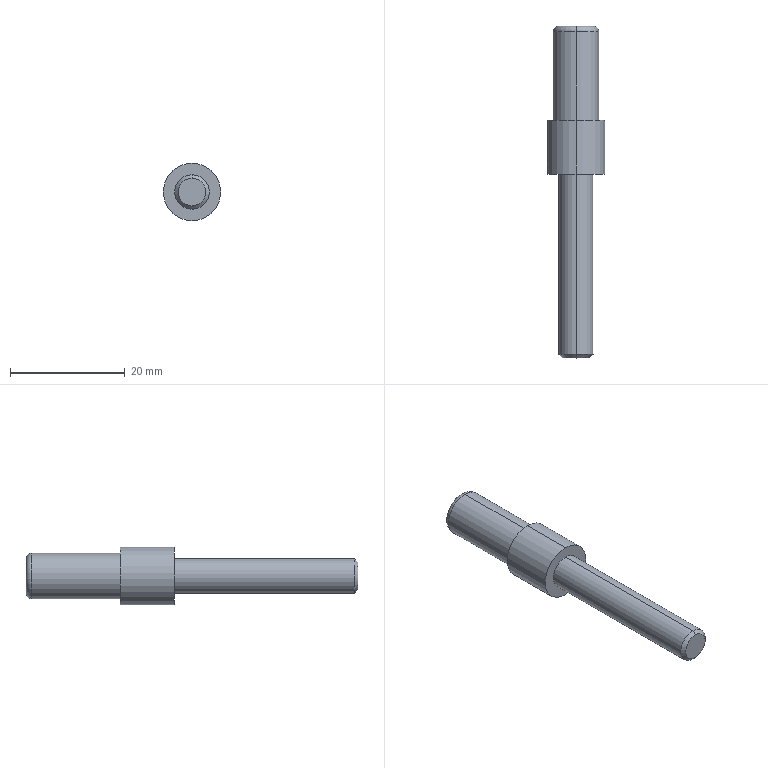Part | SolidWorks | features RefAxis 3, 3DProfileFeature 1, ICE 1, Revolution 1 | 1 solid | 21 faces | box 10 x 57.8 x 10 mm | volume 2436 mm3 | plane 11 | cylinder 6 | cone 2 | torus 2 | commonest cylinder face diameters 6 x2 8 x2 10 x2
STEP:
#1=CARTESIAN_POINT('',(0.,-32.,2.386));
#2=VERTEX_POINT('',#1);
#3=CARTESIAN_POINT('',(0.,-32.,-2.386));
#4=VERTEX_POINT('',#3);
#5=CARTESIAN_POINT('',(0.,-32.,0.));
#6=DIRECTION('',(0.,1.,0.));
#7=DIRECTION('',(0.,0.,1.));
#8=AXIS2_PLACEMENT_3D('',#5,#6,#7);
#9=CIRCLE('',#8,2.386);
#10=EDGE_CURVE('',#2,#4,#9,.T.);
#11=ORIENTED_EDGE('',*,*,#10,.T.);
#12=CARTESIAN_POINT('',(0.,-31.386,-3.));
#13=VERTEX_POINT('',#12);
#14=CARTESIAN_POINT('',(0.,-32.,-2.386));
#15=DIRECTION('',(0.,0.7071,-0.7071));
#16=VECTOR('',#15,1000.);
#17=LINE('',#14,#16);
#18=EDGE_CURVE('',#4,#13,#17,.T.);
#19=ORIENTED_EDGE('',*,*,#18,.T.);
#20=CARTESIAN_POINT('',(0.,-31.386,3.));
#21=VERTEX_POINT('',#20);
#22=CARTESIAN_POINT('',(0.,-31.386,0.));
#23=DIRECTION('',(0.,1.,0.));
#24=DIRECTION('',(0.,0.,1.));
#25=AXIS2_PLACEMENT_3D('',#22,#23,#24);
#26=CIRCLE('',#25,3.);
#27=EDGE_CURVE('',#21,#13,#26,.T.);
#28=ORIENTED_EDGE('',*,*,#27,.F.);
#29=CARTESIAN_POINT('',(0.,-32.,2.386));
#30=DIRECTION('',(0.,0.7071,0.7071));
#31=VECTOR('',#30,1000.);
#32=LINE('',#29,#31);
#33=EDGE_CURVE('',#2,#21,#32,.T.);
#34=ORIENTED_EDGE('',*,*,#33,.F.);
#35=EDGE_LOOP('',(#11,#19,#28,#34));
#36=FACE_OUTER_BOUND('',#35,.T.);
#37=CARTESIAN_POINT('',(0.,-32.,0.));
#38=DIRECTION('',(0.,1.,0.));
#39=DIRECTION('',(0.,0.,1.));
#40=AXIS2_PLACEMENT_3D('',#37,#38,#39);
#41=CONICAL_SURFACE('',#40,2.386,0.7854);
#42=ADVANCED_FACE('',(#36),#41,.T.);
#43=ORIENTED_EDGE('',*,*,#27,.T.);
#44=CARTESIAN_POINT('',(0.,0.,-3.));
#45=VERTEX_POINT('',#44);
#46=CARTESIAN_POINT('',(0.,-32.,-3.));
#47=DIRECTION('',(0.,1.,0.));
#48=VECTOR('',#47,1000.);
#49=LINE('',#46,#48);
#50=EDGE_CURVE('',#13,#45,#49,.T.);
#51=ORIENTED_EDGE('',*,*,#50,.T.);
#52=CARTESIAN_POINT('',(0.,0.,3.));
#53=VERTEX_POINT('',#52);
#54=CARTESIAN_POINT('',(0.,0.,0.));
#55=DIRECTION('',(0.,1.,0.));
#56=DIRECTION('',(0.,0.,1.));
#57=AXIS2_PLACEMENT_3D('',#54,#55,#56);
#58=CIRCLE('',#57,3.);
#59=EDGE_CURVE('',#53,#45,#58,.T.);
#60=ORIENTED_EDGE('',*,*,#59,.F.);
#61=CARTESIAN_POINT('',(0.,-32.,3.));
#62=DIRECTION('',(0.,1.,0.));
#63=VECTOR('',#62,1000.);
#64=LINE('',#61,#63);
#65=EDGE_CURVE('',#21,#53,#64,.T.);
#66=ORIENTED_EDGE('',*,*,#65,.F.);
#67=EDGE_LOOP('',(#43,#51,#60,#66));
#68=FACE_OUTER_BOUND('',#67,.T.);
#69=CARTESIAN_POINT('',(0.,-32.,0.));
#70=DIRECTION('',(0.,1.,0.));
#71=DIRECTION('',(0.,0.,1.));
#72=AXIS2_PLACEMENT_3D('',#69,#70,#71);
#73=CYLINDRICAL_SURFACE('',#72,3.);
#74=ADVANCED_FACE('',(#68),#73,.T.);
#75=CARTESIAN_POINT('',(0.,0.,5.));
#76=VERTEX_POINT('',#75);
#77=CARTESIAN_POINT('',(0.,0.,-5.));
#78=VERTEX_POINT('',#77);
#79=CARTESIAN_POINT('',(0.,0.,0.));
#80=DIRECTION('',(0.,1.,0.));
#81=DIRECTION('',(0.,0.,1.));
#82=AXIS2_PLACEMENT_3D('',#79,#80,#81);
#83=CIRCLE('',#82,5.);
#84=EDGE_CURVE('',#76,#78,#83,.T.);
#85=ORIENTED_EDGE('',*,*,#84,.T.);
#86=CARTESIAN_POINT('',(0.,9.4,-5.));
#87=VERTEX_POINT('',#86);
#88=CARTESIAN_POINT('',(0.,-32.,-5.));
#89=DIRECTION('',(0.,1.,0.));
#90=VECTOR('',#89,1000.);
#91=LINE('',#88,#90);
#92=EDGE_CURVE('',#78,#87,#91,.T.);
#93=ORIENTED_EDGE('',*,*,#92,.T.);
#94=CARTESIAN_POINT('',(0.,9.4,5.));
#95=VERTEX_POINT('',#94);
#96=CARTESIAN_POINT('',(0.,9.4,0.));
#97=DIRECTION('',(0.,1.,0.));
#98=DIRECTION('',(0.,0.,1.));
#99=AXIS2_PLACEMENT_3D('',#96,#97,#98);
#100=CIRCLE('',#99,5.);
#101=EDGE_CURVE('',#95,#87,#100,.T.);
#102=ORIENTED_EDGE('',*,*,#101,.F.);
#103=CARTESIAN_POINT('',(0.,-32.,5.));
#104=DIRECTION('',(0.,1.,0.));
#105=VECTOR('',#104,1000.);
#106=LINE('',#103,#105);
#107=EDGE_CURVE('',#76,#95,#106,.T.);
#108=ORIENTED_EDGE('',*,*,#107,.F.);
#109=EDGE_LOOP('',(#85,#93,#102,#108));
#110=FACE_OUTER_BOUND('',#109,.T.);
#111=CARTESIAN_POINT('',(0.,-32.,0.));
#112=DIRECTION('',(0.,1.,0.));
#113=DIRECTION('',(0.,0.,1.));
#114=AXIS2_PLACEMENT_3D('',#111,#112,#113);
#115=CYLINDRICAL_SURFACE('',#114,5.);
#116=ADVANCED_FACE('',(#110),#115,.T.);
#117=CARTESIAN_POINT('',(0.,9.4,4.));
#118=VERTEX_POINT('',#117);
#119=CARTESIAN_POINT('',(0.,9.4,-4.));
#120=VERTEX_POINT('',#119);
#121=CARTESIAN_POINT('',(0.,9.4,0.));
#122=DIRECTION('',(0.,1.,0.));
#123=DIRECTION('',(0.,0.,1.));
#124=AXIS2_PLACEMENT_3D('',#121,#122,#123);
#125=CIRCLE('',#124,4.);
#126=EDGE_CURVE('',#118,#120,#125,.T.);
#127=ORIENTED_EDGE('',*,*,#126,.T.);
#128=CARTESIAN_POINT('',(0.,24.8,-4.));
#129=VERTEX_POINT('',#128);
#130=CARTESIAN_POINT('',(0.,-32.,-4.));
#131=DIRECTION('',(0.,1.,0.));
#132=VECTOR('',#131,1000.);
#133=LINE('',#130,#132);
#134=EDGE_CURVE('',#120,#129,#133,.T.);
#135=ORIENTED_EDGE('',*,*,#134,.T.);
#136=CARTESIAN_POINT('',(0.,24.8,4.));
#137=VERTEX_POINT('',#136);
#138=CARTESIAN_POINT('',(0.,24.8,0.));
#139=DIRECTION('',(0.,1.,0.));
#140=DIRECTION('',(0.,0.,1.));
#141=AXIS2_PLACEMENT_3D('',#138,#139,#140);
#142=CIRCLE('',#141,4.);
#143=EDGE_CURVE('',#137,#129,#142,.T.);
#144=ORIENTED_EDGE('',*,*,#143,.F.);
#145=CARTESIAN_POINT('',(0.,-32.,4.));
#146=DIRECTION('',(0.,1.,0.));
#147=VECTOR('',#146,1000.);
#148=LINE('',#145,#147);
#149=EDGE_CURVE('',#118,#137,#148,.T.);
#150=ORIENTED_EDGE('',*,*,#149,.F.);
#151=EDGE_LOOP('',(#127,#135,#144,#150));
#152=FACE_OUTER_BOUND('',#151,.T.);
#153=CARTESIAN_POINT('',(0.,-32.,0.));
#154=DIRECTION('',(0.,1.,0.));
#155=DIRECTION('',(0.,0.,1.));
#156=AXIS2_PLACEMENT_3D('',#153,#154,#155);
#157=CYLINDRICAL_SURFACE('',#156,4.);
#158=ADVANCED_FACE('',(#152),#157,.T.);
#159=ORIENTED_EDGE('',*,*,#143,.T.);
#160=CARTESIAN_POINT('',(0.,25.8,-3.));
#161=VERTEX_POINT('',#160);
#162=CARTESIAN_POINT('',(0.,24.8,-3.));
#163=DIRECTION('',(1.,0.,0.));
#164=DIRECTION('',(0.,0.,-1.));
#165=AXIS2_PLACEMENT_3D('',#162,#163,#164);
#166=CIRCLE('',#165,1.);
#167=EDGE_CURVE('',#129,#161,#166,.T.);
#168=ORIENTED_EDGE('',*,*,#167,.T.);
#169=CARTESIAN_POINT('',(0.,25.8,3.));
#170=VERTEX_POINT('',#169);
#171=CARTESIAN_POINT('',(0.,25.8,0.));
#172=DIRECTION('',(0.,1.,0.));
#173=DIRECTION('',(0.,0.,1.));
#174=AXIS2_PLACEMENT_3D('',#171,#172,#173);
#175=CIRCLE('',#174,3.);
#176=EDGE_CURVE('',#170,#161,#175,.T.);
#177=ORIENTED_EDGE('',*,*,#176,.F.);
#178=CARTESIAN_POINT('',(0.,24.8,3.));
#179=DIRECTION('',(-1.,0.,0.));
#180=DIRECTION('',(0.,0.,1.));
#181=AXIS2_PLACEMENT_3D('',#178,#179,#180);
#182=CIRCLE('',#181,1.);
#183=EDGE_CURVE('',#137,#170,#182,.T.);
#184=ORIENTED_EDGE('',*,*,#183,.F.);
#185=EDGE_LOOP('',(#159,#168,#177,#184));
#186=FACE_OUTER_BOUND('',#185,.T.);
#187=CARTESIAN_POINT('',(0.,24.8,0.));
#188=DIRECTION('',(0.,1.,0.));
#189=DIRECTION('',(0.,0.,1.));
#190=AXIS2_PLACEMENT_3D('',#187,#188,#189);
#191=TOROIDAL_SURFACE('',#190,3.,1.);
#192=ADVANCED_FACE('',(#186),#191,.T.);
#193=CARTESIAN_POINT('',(-1.5,25.8,0.866));
#194=VERTEX_POINT('',#193);
#195=CARTESIAN_POINT('',(-1.5,25.8,-0.866));
#196=VERTEX_POINT('',#195);
#197=CARTESIAN_POINT('',(-1.5,25.8,0.));
#198=DIRECTION('',(0.,0.,-1.));
#199=VECTOR('',#198,1000.);
#200=LINE('',#197,#199);
#201=EDGE_CURVE('',#194,#196,#200,.T.);
#202=ORIENTED_EDGE('',*,*,#201,.T.);
#203=CARTESIAN_POINT('',(0.,25.8,-1.732));
#204=VERTEX_POINT('',#203);
#205=CARTESIAN_POINT('',(-0.75,25.8,-1.299));
#206=DIRECTION('',(0.866,0.,-0.5));
#207=VECTOR('',#206,1000.);
#208=LINE('',#205,#207);
#209=EDGE_CURVE('',#196,#204,#208,.T.);
#210=ORIENTED_EDGE('',*,*,#209,.T.);
#211=CARTESIAN_POINT('',(1.5,25.8,-0.866));
#212=VERTEX_POINT('',#211);
#213=CARTESIAN_POINT('',(0.75,25.8,-1.299));
#214=DIRECTION('',(0.866,0.,0.5));
#215=VECTOR('',#214,1000.);
#216=LINE('',#213,#215);
#217=EDGE_CURVE('',#204,#212,#216,.T.);
#218=ORIENTED_EDGE('',*,*,#217,.T.);
#219=CARTESIAN_POINT('',(1.5,25.8,0.866));
#220=VERTEX_POINT('',#219);
#221=CARTESIAN_POINT('',(1.5,25.8,0.));
#222=DIRECTION('',(0.,0.,1.));
#223=VECTOR('',#222,1000.);
#224=LINE('',#221,#223);
#225=EDGE_CURVE('',#212,#220,#224,.T.);
#226=ORIENTED_EDGE('',*,*,#225,.T.);
#227=CARTESIAN_POINT('',(0.,25.8,1.732));
#228=VERTEX_POINT('',#227);
#229=CARTESIAN_POINT('',(0.75,25.8,1.299));
#230=DIRECTION('',(-0.866,0.,0.5));
#231=VECTOR('',#230,1000.);
#232=LINE('',#229,#231);
#233=EDGE_CURVE('',#220,#228,#232,.T.);
#234=ORIENTED_EDGE('',*,*,#233,.T.);
#235=CARTESIAN_POINT('',(-0.75,25.8,1.299));
#236=DIRECTION('',(-0.866,0.,-0.5));
#237=VECTOR('',#236,1000.);
#238=LINE('',#235,#237);
#239=EDGE_CURVE('',#228,#194,#238,.T.);
#240=ORIENTED_EDGE('',*,*,#239,.T.);
#241=EDGE_LOOP('',(#202,#210,#218,#226,#234,#240));
#242=FACE_BOUND('',#241,.T.);
#243=ORIENTED_EDGE('',*,*,#176,.T.);
#244=CARTESIAN_POINT('',(0.,25.8,0.));
#245=DIRECTION('',(0.,1.,0.));
#246=DIRECTION('',(0.,0.,1.));
#247=AXIS2_PLACEMENT_3D('',#244,#245,#246);
#248=CIRCLE('',#247,3.);
#249=EDGE_CURVE('',#161,#170,#248,.T.);
#250=ORIENTED_EDGE('',*,*,#249,.T.);
#251=EDGE_LOOP('',(#243,#250));
#252=FACE_OUTER_BOUND('',#251,.T.);
#253=CARTESIAN_POINT('',(0.,25.8,0.));
#254=DIRECTION('',(0.,-1.,0.));
#255=DIRECTION('',(0.,0.,-1.));
#256=AXIS2_PLACEMENT_3D('',#253,#254,#255);
#257=PLANE('',#256);
#258=ADVANCED_FACE('',(#242,#252),#257,.F.);
#259=ORIENTED_EDGE('',*,*,#167,.F.);
#260=CARTESIAN_POINT('',(0.,24.8,0.));
#261=DIRECTION('',(0.,1.,0.));
#262=DIRECTION('',(0.,0.,1.));
#263=AXIS2_PLACEMENT_3D('',#260,#261,#262);
#264=CIRCLE('',#263,4.);
#265=EDGE_CURVE('',#129,#137,#264,.T.);
#266=ORIENTED_EDGE('',*,*,#265,.T.);
#267=ORIENTED_EDGE('',*,*,#183,.T.);
#268=ORIENTED_EDGE('',*,*,#249,.F.);
#269=EDGE_LOOP('',(#259,#266,#267,#268));
#270=FACE_OUTER_BOUND('',#269,.T.);
#271=CARTESIAN_POINT('',(0.,24.8,0.));
#272=DIRECTION('',(0.,1.,0.));
#273=DIRECTION('',(0.,0.,1.));
#274=AXIS2_PLACEMENT_3D('',#271,#272,#273);
#275=TOROIDAL_SURFACE('',#274,3.,1.);
#276=ADVANCED_FACE('',(#270),#275,.T.);
#277=ORIENTED_EDGE('',*,*,#134,.F.);
#278=CARTESIAN_POINT('',(0.,9.4,0.));
#279=DIRECTION('',(0.,1.,0.));
#280=DIRECTION('',(0.,0.,1.));
#281=AXIS2_PLACEMENT_3D('',#278,#279,#280);
#282=CIRCLE('',#281,4.);
#283=EDGE_CURVE('',#120,#118,#282,.T.);
#284=ORIENTED_EDGE('',*,*,#283,.T.);
#285=ORIENTED_EDGE('',*,*,#149,.T.);
#286=ORIENTED_EDGE('',*,*,#265,.F.);
#287=EDGE_LOOP('',(#277,#284,#285,#286));
#288=FACE_OUTER_BOUND('',#287,.T.);
#289=CARTESIAN_POINT('',(0.,-32.,0.));
#290=DIRECTION('',(0.,1.,0.));
#291=DIRECTION('',(0.,0.,1.));
#292=AXIS2_PLACEMENT_3D('',#289,#290,#291);
#293=CYLINDRICAL_SURFACE('',#292,4.);
#294=ADVANCED_FACE('',(#288),#293,.T.);
#295=ORIENTED_EDGE('',*,*,#126,.F.);
#296=ORIENTED_EDGE('',*,*,#283,.F.);
#297=EDGE_LOOP('',(#295,#296));
#298=FACE_BOUND('',#297,.T.);
#299=ORIENTED_EDGE('',*,*,#101,.T.);
#300=CARTESIAN_POINT('',(0.,9.4,0.));
#301=DIRECTION('',(0.,1.,0.));
#302=DIRECTION('',(0.,0.,1.));
#303=AXIS2_PLACEMENT_3D('',#300,#301,#302);
#304=CIRCLE('',#303,5.);
#305=EDGE_CURVE('',#87,#95,#304,.T.);
#306=ORIENTED_EDGE('',*,*,#305,.T.);
#307=EDGE_LOOP('',(#299,#306));
#308=FACE_OUTER_BOUND('',#307,.T.);
#309=CARTESIAN_POINT('',(4.,9.4,0.));
#310=DIRECTION('',(0.,-1.,0.));
#311=DIRECTION('',(0.,0.,-1.));
#312=AXIS2_PLACEMENT_3D('',#309,#310,#311);
#313=PLANE('',#312);
#314=ADVANCED_FACE('',(#298,#308),#313,.F.);
#315=ORIENTED_EDGE('',*,*,#92,.F.);
#316=CARTESIAN_POINT('',(0.,0.,0.));
#317=DIRECTION('',(0.,1.,0.));
#318=DIRECTION('',(0.,0.,1.));
#319=AXIS2_PLACEMENT_3D('',#316,#317,#318);
#320=CIRCLE('',#319,5.);
#321=EDGE_CURVE('',#78,#76,#320,.T.);
#322=ORIENTED_EDGE('',*,*,#321,.T.);
#323=ORIENTED_EDGE('',*,*,#107,.T.);
#324=ORIENTED_EDGE('',*,*,#305,.F.);
#325=EDGE_LOOP('',(#315,#322,#323,#324));
#326=FACE_OUTER_BOUND('',#325,.T.);
#327=CARTESIAN_POINT('',(0.,-32.,0.));
#328=DIRECTION('',(0.,1.,0.));
#329=DIRECTION('',(0.,0.,1.));
#330=AXIS2_PLACEMENT_3D('',#327,#328,#329);
#331=CYLINDRICAL_SURFACE('',#330,5.);
#332=ADVANCED_FACE('',(#326),#331,.T.);
#333=ORIENTED_EDGE('',*,*,#84,.F.);
#334=ORIENTED_EDGE('',*,*,#321,.F.);
#335=EDGE_LOOP('',(#333,#334));
#336=FACE_OUTER_BOUND('',#335,.T.);
#337=ORIENTED_EDGE('',*,*,#59,.T.);
#338=CARTESIAN_POINT('',(0.,0.,0.));
#339=DIRECTION('',(0.,1.,0.));
#340=DIRECTION('',(0.,0.,1.));
#341=AXIS2_PLACEMENT_3D('',#338,#339,#340);
#342=CIRCLE('',#341,3.);
#343=EDGE_CURVE('',#45,#53,#342,.T.);
#344=ORIENTED_EDGE('',*,*,#343,.T.);
#345=EDGE_LOOP('',(#337,#344));
#346=FACE_BOUND('',#345,.T.);
#347=CARTESIAN_POINT('',(5.,0.,0.));
#348=DIRECTION('',(0.,1.,0.));
#349=DIRECTION('',(0.,0.,1.));
#350=AXIS2_PLACEMENT_3D('',#347,#348,#349);
#351=PLANE('',#350);
#352=ADVANCED_FACE('',(#336,#346),#351,.F.);
#353=ORIENTED_EDGE('',*,*,#50,.F.);
#354=CARTESIAN_POINT('',(0.,-31.386,0.));
#355=DIRECTION('',(0.,1.,0.));
#356=DIRECTION('',(0.,0.,1.));
#357=AXIS2_PLACEMENT_3D('',#354,#355,#356);
#358=CIRCLE('',#357,3.);
#359=EDGE_CURVE('',#13,#21,#358,.T.);
#360=ORIENTED_EDGE('',*,*,#359,.T.);
#361=ORIENTED_EDGE('',*,*,#65,.T.);
#362=ORIENTED_EDGE('',*,*,#343,.F.);
#363=EDGE_LOOP('',(#353,#360,#361,#362));
#364=FACE_OUTER_BOUND('',#363,.T.);
#365=CARTESIAN_POINT('',(0.,-32.,0.));
#366=DIRECTION('',(0.,1.,0.));
#367=DIRECTION('',(0.,0.,1.));
#368=AXIS2_PLACEMENT_3D('',#365,#366,#367);
#369=CYLINDRICAL_SURFACE('',#368,3.);
#370=ADVANCED_FACE('',(#364),#369,.T.);
#371=ORIENTED_EDGE('',*,*,#18,.F.);
#372=CARTESIAN_POINT('',(0.,-32.,0.));
#373=DIRECTION('',(0.,1.,0.));
#374=DIRECTION('',(0.,0.,1.));
#375=AXIS2_PLACEMENT_3D('',#372,#373,#374);
#376=CIRCLE('',#375,2.386);
#377=EDGE_CURVE('',#4,#2,#376,.T.);
#378=ORIENTED_EDGE('',*,*,#377,.T.);
#379=ORIENTED_EDGE('',*,*,#33,.T.);
#380=ORIENTED_EDGE('',*,*,#359,.F.);
#381=EDGE_LOOP('',(#371,#378,#379,#380));
#382=FACE_OUTER_BOUND('',#381,.T.);
#383=CARTESIAN_POINT('',(0.,-32.,0.));
#384=DIRECTION('',(0.,1.,0.));
#385=DIRECTION('',(0.,0.,1.));
#386=AXIS2_PLACEMENT_3D('',#383,#384,#385);
#387=CONICAL_SURFACE('',#386,2.386,0.7854);
#388=ADVANCED_FACE('',(#382),#387,.T.);
#389=ORIENTED_EDGE('',*,*,#10,.F.);
#390=ORIENTED_EDGE('',*,*,#377,.F.);
#391=EDGE_LOOP('',(#389,#390));
#392=FACE_OUTER_BOUND('',#391,.T.);
#393=CARTESIAN_POINT('',(2.386,-32.,0.));
#394=DIRECTION('',(0.,1.,0.));
#395=DIRECTION('',(0.,0.,1.));
#396=AXIS2_PLACEMENT_3D('',#393,#394,#395);
#397=PLANE('',#396);
#398=ADVANCED_FACE('',(#392),#397,.F.);
#399=CARTESIAN_POINT('',(-1.5,22.8,-0.866));
#400=VERTEX_POINT('',#399);
#401=CARTESIAN_POINT('',(-1.5,22.8,-0.866));
#402=DIRECTION('',(0.,1.,0.));
#403=VECTOR('',#402,1000.);
#404=LINE('',#401,#403);
#405=EDGE_CURVE('',#400,#196,#404,.T.);
#406=ORIENTED_EDGE('',*,*,#405,.F.);
#407=CARTESIAN_POINT('',(0.,22.8,-1.732));
#408=VERTEX_POINT('',#407);
#409=CARTESIAN_POINT('',(0.,22.8,-1.732));
#410=DIRECTION('',(-0.866,0.,0.5));
#411=VECTOR('',#410,1000.);
#412=LINE('',#409,#411);
#413=EDGE_CURVE('',#408,#400,#412,.T.);
#414=ORIENTED_EDGE('',*,*,#413,.F.);
#415=CARTESIAN_POINT('',(0.,22.8,-1.732));
#416=DIRECTION('',(0.,1.,0.));
#417=VECTOR('',#416,1000.);
#418=LINE('',#415,#417);
#419=EDGE_CURVE('',#408,#204,#418,.T.);
#420=ORIENTED_EDGE('',*,*,#419,.T.);
#421=ORIENTED_EDGE('',*,*,#209,.F.);
#422=EDGE_LOOP('',(#406,#414,#420,#421));
#423=FACE_OUTER_BOUND('',#422,.T.);
#424=CARTESIAN_POINT('',(0.,22.8,-1.732));
#425=DIRECTION('',(-0.5,0.,-0.866));
#426=DIRECTION('',(-0.866,0.,0.5));
#427=AXIS2_PLACEMENT_3D('',#424,#425,#426);
#428=PLANE('',#427);
#429=ADVANCED_FACE('',(#423),#428,.F.);
#430=ORIENTED_EDGE('',*,*,#419,.F.);
#431=CARTESIAN_POINT('',(1.5,22.8,-0.866));
#432=VERTEX_POINT('',#431);
#433=CARTESIAN_POINT('',(1.5,22.8,-0.866));
#434=DIRECTION('',(-0.866,0.,-0.5));
#435=VECTOR('',#434,1000.);
#436=LINE('',#433,#435);
#437=EDGE_CURVE('',#432,#408,#436,.T.);
#438=ORIENTED_EDGE('',*,*,#437,.F.);
#439=CARTESIAN_POINT('',(1.5,22.8,-0.866));
#440=DIRECTION('',(0.,1.,0.));
#441=VECTOR('',#440,1000.);
#442=LINE('',#439,#441);
#443=EDGE_CURVE('',#432,#212,#442,.T.);
#444=ORIENTED_EDGE('',*,*,#443,.T.);
#445=ORIENTED_EDGE('',*,*,#217,.F.);
#446=EDGE_LOOP('',(#430,#438,#444,#445));
#447=FACE_OUTER_BOUND('',#446,.T.);
#448=CARTESIAN_POINT('',(1.5,22.8,-0.866));
#449=DIRECTION('',(0.5,0.,-0.866));
#450=DIRECTION('',(-0.866,0.,-0.5));
#451=AXIS2_PLACEMENT_3D('',#448,#449,#450);
#452=PLANE('',#451);
#453=ADVANCED_FACE('',(#447),#452,.F.);
#454=ORIENTED_EDGE('',*,*,#443,.F.);
#455=CARTESIAN_POINT('',(1.5,22.8,0.866));
#456=VERTEX_POINT('',#455);
#457=CARTESIAN_POINT('',(1.5,22.8,0.866));
#458=DIRECTION('',(0.,0.,-1.));
#459=VECTOR('',#458,1000.);
#460=LINE('',#457,#459);
#461=EDGE_CURVE('',#456,#432,#460,.T.);
#462=ORIENTED_EDGE('',*,*,#461,.F.);
#463=CARTESIAN_POINT('',(1.5,22.8,0.866));
#464=DIRECTION('',(0.,1.,0.));
#465=VECTOR('',#464,1000.);
#466=LINE('',#463,#465);
#467=EDGE_CURVE('',#456,#220,#466,.T.);
#468=ORIENTED_EDGE('',*,*,#467,.T.);
#469=ORIENTED_EDGE('',*,*,#225,.F.);
#470=EDGE_LOOP('',(#454,#462,#468,#469));
#471=FACE_OUTER_BOUND('',#470,.T.);
#472=CARTESIAN_POINT('',(1.5,22.8,0.866));
#473=DIRECTION('',(1.,0.,0.));
#474=DIRECTION('',(0.,0.,-1.));
#475=AXIS2_PLACEMENT_3D('',#472,#473,#474);
#476=PLANE('',#475);
#477=ADVANCED_FACE('',(#471),#476,.F.);
#478=ORIENTED_EDGE('',*,*,#467,.F.);
#479=CARTESIAN_POINT('',(0.,22.8,1.732));
#480=VERTEX_POINT('',#479);
#481=CARTESIAN_POINT('',(0.,22.8,1.732));
#482=DIRECTION('',(0.866,0.,-0.5));
#483=VECTOR('',#482,1000.);
#484=LINE('',#481,#483);
#485=EDGE_CURVE('',#480,#456,#484,.T.);
#486=ORIENTED_EDGE('',*,*,#485,.F.);
#487=CARTESIAN_POINT('',(0.,22.8,1.732));
#488=DIRECTION('',(0.,1.,0.));
#489=VECTOR('',#488,1000.);
#490=LINE('',#487,#489);
#491=EDGE_CURVE('',#480,#228,#490,.T.);
#492=ORIENTED_EDGE('',*,*,#491,.T.);
#493=ORIENTED_EDGE('',*,*,#233,.F.);
#494=EDGE_LOOP('',(#478,#486,#492,#493));
#495=FACE_OUTER_BOUND('',#494,.T.);
#496=CARTESIAN_POINT('',(0.,22.8,1.732));
#497=DIRECTION('',(0.5,0.,0.866));
#498=DIRECTION('',(0.866,0.,-0.5));
#499=AXIS2_PLACEMENT_3D('',#496,#497,#498);
#500=PLANE('',#499);
#501=ADVANCED_FACE('',(#495),#500,.F.);
#502=ORIENTED_EDGE('',*,*,#491,.F.);
#503=CARTESIAN_POINT('',(-1.5,22.8,0.866));
#504=VERTEX_POINT('',#503);
#505=CARTESIAN_POINT('',(-1.5,22.8,0.866));
#506=DIRECTION('',(0.866,0.,0.5));
#507=VECTOR('',#506,1000.);
#508=LINE('',#505,#507);
#509=EDGE_CURVE('',#504,#480,#508,.T.);
#510=ORIENTED_EDGE('',*,*,#509,.F.);
#511=CARTESIAN_POINT('',(-1.5,22.8,0.866));
#512=DIRECTION('',(0.,1.,0.));
#513=VECTOR('',#512,1000.);
#514=LINE('',#511,#513);
#515=EDGE_CURVE('',#504,#194,#514,.T.);
#516=ORIENTED_EDGE('',*,*,#515,.T.);
#517=ORIENTED_EDGE('',*,*,#239,.F.);
#518=EDGE_LOOP('',(#502,#510,#516,#517));
#519=FACE_OUTER_BOUND('',#518,.T.);
#520=CARTESIAN_POINT('',(-1.5,22.8,0.866));
#521=DIRECTION('',(-0.5,0.,0.866));
#522=DIRECTION('',(0.866,0.,0.5));
#523=AXIS2_PLACEMENT_3D('',#520,#521,#522);
#524=PLANE('',#523);
#525=ADVANCED_FACE('',(#519),#524,.F.);
#526=ORIENTED_EDGE('',*,*,#515,.F.);
#527=CARTESIAN_POINT('',(-1.5,22.8,-0.866));
#528=DIRECTION('',(0.,0.,1.));
#529=VECTOR('',#528,1000.);
#530=LINE('',#527,#529);
#531=EDGE_CURVE('',#400,#504,#530,.T.);
#532=ORIENTED_EDGE('',*,*,#531,.F.);
#533=ORIENTED_EDGE('',*,*,#405,.T.);
#534=ORIENTED_EDGE('',*,*,#201,.F.);
#535=EDGE_LOOP('',(#526,#532,#533,#534));
#536=FACE_OUTER_BOUND('',#535,.T.);
#537=CARTESIAN_POINT('',(-1.5,22.8,-0.866));
#538=DIRECTION('',(-1.,0.,0.));
#539=DIRECTION('',(0.,0.,1.));
#540=AXIS2_PLACEMENT_3D('',#537,#538,#539);
#541=PLANE('',#540);
#542=ADVANCED_FACE('',(#536),#541,.F.);
#543=ORIENTED_EDGE('',*,*,#413,.T.);
#544=ORIENTED_EDGE('',*,*,#531,.T.);
#545=ORIENTED_EDGE('',*,*,#509,.T.);
#546=ORIENTED_EDGE('',*,*,#485,.T.);
#547=ORIENTED_EDGE('',*,*,#461,.T.);
#548=ORIENTED_EDGE('',*,*,#437,.T.);
#549=EDGE_LOOP('',(#543,#544,#545,#546,#547,#548));
#550=FACE_OUTER_BOUND('',#549,.T.);
#551=CARTESIAN_POINT('',(0.,22.8,0.));
#552=DIRECTION('',(0.,1.,0.));
#553=DIRECTION('',(0.,0.,1.));
#554=AXIS2_PLACEMENT_3D('',#551,#552,#553);
#555=PLANE('',#554);
#556=ADVANCED_FACE('',(#550),#555,.T.);
#557=CLOSED_SHELL('',(#42,#74,#116,#158,#192,#258,#276,#294,#314,#332,#352,#370,#388,#398,#429,#453,#477,#501,#525,#542,#556));
#558=MANIFOLD_SOLID_BREP('',#557);
#559=CARTESIAN_POINT('',(0.,0.,0.));
#560=DIRECTION('',(0.,0.,1.));
#561=DIRECTION('',(1.,0.,0.));
#562=AXIS2_PLACEMENT_3D('',#559,#560,#561);
#563=(LENGTH_UNIT()NAMED_UNIT(*)SI_UNIT(.MILLI.,.METRE.));
#564=UNCERTAINTY_MEASURE_WITH_UNIT(LENGTH_MEASURE(0.00001),#563,'','');
#565=(NAMED_UNIT(*)PLANE_ANGLE_UNIT()SI_UNIT($,.RADIAN.));
#566=(NAMED_UNIT(*)SI_UNIT($,.STERADIAN.)SOLID_ANGLE_UNIT());
#567=(GEOMETRIC_REPRESENTATION_CONTEXT(3)GLOBAL_UNCERTAINTY_ASSIGNED_CONTEXT((#564))GLOBAL_UNIT_ASSIGNED_CONTEXT((#563,#565,#566))REPRESENTATION_CONTEXT('',''));
#568=ADVANCED_BREP_SHAPE_REPRESENTATION('',(#558,#562),#567);